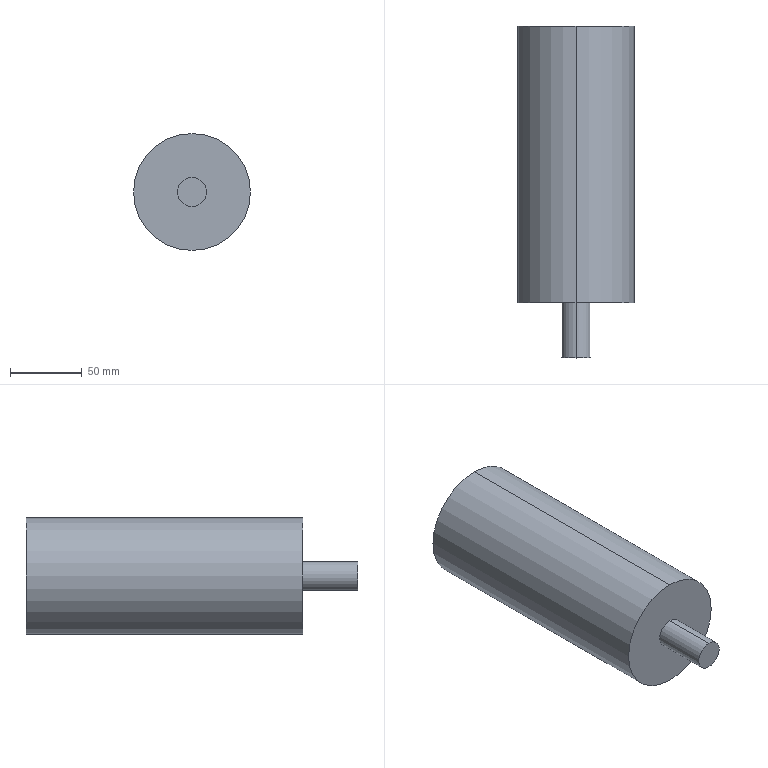Part | STEP file | 1 solid | 7 faces | box 81.521 x 231.5 x 81.521 mm | volume 1019717 mm3 | cylinder 4 | plane 3 | commonest cylinder face diameters 20.209 x2 81.521 x2
STEP:
#1=CARTESIAN_POINT('',(0.,0.,0.));
#2=DIRECTION('',(0.,0.,1.));
#3=DIRECTION('',(1.,0.,0.));
#4=AXIS2_PLACEMENT_3D('',#1,#2,#3);
#5=CARTESIAN_POINT('',(340.649,211.514,236.001));
#6=VERTEX_POINT('',#5);
#7=CARTESIAN_POINT('',(340.649,211.514,256.211));
#8=VERTEX_POINT('',#7);
#9=CARTESIAN_POINT('',(340.649,211.514,246.106));
#10=DIRECTION('',(0.,-1.,0.));
#11=DIRECTION('',(0.,0.,-1.));
#12=AXIS2_PLACEMENT_3D('',#9,#10,#11);
#13=CIRCLE('',#12,10.105);
#14=CARTESIAN_POINT('',(340.649,211.514,246.106));
#15=DIRECTION('',(0.,1.,0.));
#16=DIRECTION('',(0.,0.,1.));
#17=AXIS2_PLACEMENT_3D('',#14,#15,#16);
#18=CYLINDRICAL_SURFACE('',#17,10.105);
#19=CARTESIAN_POINT('',(3.142,0.));
#20=DIRECTION('',(-1.,0.));
#21=VECTOR('',#20,1.);
#22=LINE('',#19,#21);
#23=(GEOMETRIC_REPRESENTATION_CONTEXT(2)PARAMETRIC_REPRESENTATION_CONTEXT()REPRESENTATION_CONTEXT('',''));
#24=DEFINITIONAL_REPRESENTATION('',(#22),#23);
#25=PCURVE('',#18,#24);
#26=CARTESIAN_POINT('',(340.649,211.514,246.106));
#27=DIRECTION('',(0.,-1.,0.));
#28=DIRECTION('',(0.,0.,-1.));
#29=AXIS2_PLACEMENT_3D('',#26,#27,#28);
#30=PLANE('',#29);
#31=CARTESIAN_POINT('',(0.,0.));
#32=DIRECTION('',(1.,0.));
#33=AXIS2_PLACEMENT_2D('',#31,#32);
#34=CIRCLE('',#33,10.105);
#35=(GEOMETRIC_REPRESENTATION_CONTEXT(2)PARAMETRIC_REPRESENTATION_CONTEXT()REPRESENTATION_CONTEXT('',''));
#36=DEFINITIONAL_REPRESENTATION('',(#34),#35);
#37=PCURVE('',#30,#36);
#38=SURFACE_CURVE('',#13,(#25,#37),.PCURVE_S1.);
#39=EDGE_CURVE('',#6,#8,#38,.T.);
#40=ORIENTED_EDGE('',*,*,#39,.F.);
#41=CARTESIAN_POINT('',(340.649,250.014,236.001));
#42=VERTEX_POINT('',#41);
#43=CARTESIAN_POINT('',(340.649,211.514,236.001));
#44=DIRECTION('',(0.,1.,0.));
#45=VECTOR('',#44,1.);
#46=LINE('',#43,#45);
#47=CARTESIAN_POINT('',(3.142,0.));
#48=DIRECTION('',(0.,1.));
#49=VECTOR('',#48,1.);
#50=LINE('',#47,#49);
#51=(GEOMETRIC_REPRESENTATION_CONTEXT(2)PARAMETRIC_REPRESENTATION_CONTEXT()REPRESENTATION_CONTEXT('',''));
#52=DEFINITIONAL_REPRESENTATION('',(#50),#51);
#53=PCURVE('',#18,#52);
#54=CARTESIAN_POINT('',(340.649,211.514,246.106));
#55=DIRECTION('',(0.,1.,0.));
#56=DIRECTION('',(0.,0.,1.));
#57=AXIS2_PLACEMENT_3D('',#54,#55,#56);
#58=CYLINDRICAL_SURFACE('',#57,10.105);
#59=CARTESIAN_POINT('',(3.142,0.));
#60=DIRECTION('',(0.,1.));
#61=VECTOR('',#60,1.);
#62=LINE('',#59,#61);
#63=(GEOMETRIC_REPRESENTATION_CONTEXT(2)PARAMETRIC_REPRESENTATION_CONTEXT()REPRESENTATION_CONTEXT('',''));
#64=DEFINITIONAL_REPRESENTATION('',(#62),#63);
#65=PCURVE('',#58,#64);
#66=SURFACE_CURVE('',#46,(#53,#65),.PCURVE_S1.);
#67=EDGE_CURVE('',#6,#42,#66,.T.);
#68=ORIENTED_EDGE('',*,*,#67,.T.);
#69=CARTESIAN_POINT('',(340.649,250.014,256.211));
#70=VERTEX_POINT('',#69);
#71=CARTESIAN_POINT('',(340.649,250.014,246.106));
#72=DIRECTION('',(0.,-1.,0.));
#73=DIRECTION('',(0.,0.,1.));
#74=AXIS2_PLACEMENT_3D('',#71,#72,#73);
#75=CIRCLE('',#74,10.105);
#76=CARTESIAN_POINT('',(6.283,38.5));
#77=DIRECTION('',(-1.,0.));
#78=VECTOR('',#77,1.);
#79=LINE('',#76,#78);
#80=(GEOMETRIC_REPRESENTATION_CONTEXT(2)PARAMETRIC_REPRESENTATION_CONTEXT()REPRESENTATION_CONTEXT('',''));
#81=DEFINITIONAL_REPRESENTATION('',(#79),#80);
#82=PCURVE('',#18,#81);
#83=CARTESIAN_POINT('',(340.649,250.014,246.106));
#84=DIRECTION('',(0.,1.,0.));
#85=DIRECTION('',(0.,0.,1.));
#86=AXIS2_PLACEMENT_3D('',#83,#84,#85);
#87=PLANE('',#86);
#88=CARTESIAN_POINT('',(10.105,0.));
#89=CARTESIAN_POINT('',(10.105,-17.502));
#90=CARTESIAN_POINT('',(-5.052,-8.751));
#91=CARTESIAN_POINT('',(-20.209,0.));
#92=CARTESIAN_POINT('',(-5.052,8.751));
#93=CARTESIAN_POINT('',(10.105,17.502));
#94=CARTESIAN_POINT('',(10.105,0.));
#95=(BOUNDED_CURVE()B_SPLINE_CURVE(2,(#88,#89,#90,#91,#92,#93,#94),.UNSPECIFIED.,.T.,.F.)B_SPLINE_CURVE_WITH_KNOTS((1,2,2,2,2,1),(-2.094,0.,2.094,4.189,6.283,8.378),.UNSPECIFIED.)CURVE()GEOMETRIC_REPRESENTATION_ITEM()RATIONAL_B_SPLINE_CURVE((1.,0.5,1.,0.5,1.,0.5,1.))REPRESENTATION_ITEM(''));
#96=(GEOMETRIC_REPRESENTATION_CONTEXT(2)PARAMETRIC_REPRESENTATION_CONTEXT()REPRESENTATION_CONTEXT('',''));
#97=DEFINITIONAL_REPRESENTATION('',(#95),#96);
#98=PCURVE('',#87,#97);
#99=SURFACE_CURVE('',#75,(#82,#98),.PCURVE_S1.);
#100=EDGE_CURVE('',#42,#70,#99,.T.);
#101=ORIENTED_EDGE('',*,*,#100,.T.);
#102=CARTESIAN_POINT('',(340.649,211.514,256.211));
#103=DIRECTION('',(0.,1.,0.));
#104=VECTOR('',#103,1.);
#105=LINE('',#102,#104);
#106=CARTESIAN_POINT('',(0.,0.));
#107=DIRECTION('',(0.,1.));
#108=VECTOR('',#107,1.);
#109=LINE('',#106,#108);
#110=(GEOMETRIC_REPRESENTATION_CONTEXT(2)PARAMETRIC_REPRESENTATION_CONTEXT()REPRESENTATION_CONTEXT('',''));
#111=DEFINITIONAL_REPRESENTATION('',(#109),#110);
#112=PCURVE('',#18,#111);
#113=CARTESIAN_POINT('',(6.283,0.));
#114=DIRECTION('',(0.,1.));
#115=VECTOR('',#114,1.);
#116=LINE('',#113,#115);
#117=(GEOMETRIC_REPRESENTATION_CONTEXT(2)PARAMETRIC_REPRESENTATION_CONTEXT()REPRESENTATION_CONTEXT('',''));
#118=DEFINITIONAL_REPRESENTATION('',(#116),#117);
#119=PCURVE('',#58,#118);
#120=SURFACE_CURVE('',#105,(#112,#119),.PCURVE_S1.);
#121=EDGE_CURVE('',#8,#70,#120,.T.);
#122=ORIENTED_EDGE('',*,*,#121,.F.);
#123=EDGE_LOOP('',(#40,#68,#101,#122));
#124=FACE_BOUND('',#123,.T.);
#125=ADVANCED_FACE('',(#124),#18,.T.);
#126=CARTESIAN_POINT('',(340.649,443.014,286.866));
#127=VERTEX_POINT('',#126);
#128=CARTESIAN_POINT('',(340.649,443.014,205.345));
#129=VERTEX_POINT('',#128);
#130=CARTESIAN_POINT('',(340.649,443.014,246.106));
#131=DIRECTION('',(0.,1.,0.));
#132=DIRECTION('',(0.,0.,1.));
#133=AXIS2_PLACEMENT_3D('',#130,#131,#132);
#134=CIRCLE('',#133,40.761);
#135=CARTESIAN_POINT('',(340.649,443.014,246.106));
#136=DIRECTION('',(0.,-1.,0.));
#137=DIRECTION('',(0.,0.,-1.));
#138=AXIS2_PLACEMENT_3D('',#135,#136,#137);
#139=CYLINDRICAL_SURFACE('',#138,40.761);
#140=CARTESIAN_POINT('',(3.142,0.));
#141=DIRECTION('',(-1.,0.));
#142=VECTOR('',#141,1.);
#143=LINE('',#140,#142);
#144=(GEOMETRIC_REPRESENTATION_CONTEXT(2)PARAMETRIC_REPRESENTATION_CONTEXT()REPRESENTATION_CONTEXT('',''));
#145=DEFINITIONAL_REPRESENTATION('',(#143),#144);
#146=PCURVE('',#139,#145);
#147=CARTESIAN_POINT('',(340.649,443.014,246.106));
#148=DIRECTION('',(0.,1.,0.));
#149=DIRECTION('',(0.,0.,1.));
#150=AXIS2_PLACEMENT_3D('',#147,#148,#149);
#151=PLANE('',#150);
#152=CARTESIAN_POINT('',(0.,0.));
#153=DIRECTION('',(1.,0.));
#154=AXIS2_PLACEMENT_2D('',#152,#153);
#155=CIRCLE('',#154,40.761);
#156=(GEOMETRIC_REPRESENTATION_CONTEXT(2)PARAMETRIC_REPRESENTATION_CONTEXT()REPRESENTATION_CONTEXT('',''));
#157=DEFINITIONAL_REPRESENTATION('',(#155),#156);
#158=PCURVE('',#151,#157);
#159=SURFACE_CURVE('',#134,(#146,#158),.PCURVE_S1.);
#160=EDGE_CURVE('',#127,#129,#159,.T.);
#161=ORIENTED_EDGE('',*,*,#160,.F.);
#162=CARTESIAN_POINT('',(340.649,250.014,286.866));
#163=VERTEX_POINT('',#162);
#164=CARTESIAN_POINT('',(340.649,443.014,286.866));
#165=DIRECTION('',(0.,-1.,0.));
#166=VECTOR('',#165,1.);
#167=LINE('',#164,#166);
#168=CARTESIAN_POINT('',(3.142,0.));
#169=DIRECTION('',(0.,1.));
#170=VECTOR('',#169,1.);
#171=LINE('',#168,#170);
#172=(GEOMETRIC_REPRESENTATION_CONTEXT(2)PARAMETRIC_REPRESENTATION_CONTEXT()REPRESENTATION_CONTEXT('',''));
#173=DEFINITIONAL_REPRESENTATION('',(#171),#172);
#174=PCURVE('',#139,#173);
#175=CARTESIAN_POINT('',(340.649,443.014,246.106));
#176=DIRECTION('',(0.,-1.,0.));
#177=DIRECTION('',(0.,0.,-1.));
#178=AXIS2_PLACEMENT_3D('',#175,#176,#177);
#179=CYLINDRICAL_SURFACE('',#178,40.761);
#180=CARTESIAN_POINT('',(3.142,0.));
#181=DIRECTION('',(0.,1.));
#182=VECTOR('',#181,1.);
#183=LINE('',#180,#182);
#184=(GEOMETRIC_REPRESENTATION_CONTEXT(2)PARAMETRIC_REPRESENTATION_CONTEXT()REPRESENTATION_CONTEXT('',''));
#185=DEFINITIONAL_REPRESENTATION('',(#183),#184);
#186=PCURVE('',#179,#185);
#187=SURFACE_CURVE('',#167,(#174,#186),.PCURVE_S1.);
#188=EDGE_CURVE('',#127,#163,#187,.T.);
#189=ORIENTED_EDGE('',*,*,#188,.T.);
#190=CARTESIAN_POINT('',(340.649,250.014,205.345));
#191=VERTEX_POINT('',#190);
#192=CARTESIAN_POINT('',(340.649,250.014,246.106));
#193=DIRECTION('',(0.,1.,0.));
#194=DIRECTION('',(0.,0.,1.));
#195=AXIS2_PLACEMENT_3D('',#192,#193,#194);
#196=CIRCLE('',#195,40.761);
#197=CARTESIAN_POINT('',(3.142,193.));
#198=DIRECTION('',(-1.,0.));
#199=VECTOR('',#198,1.);
#200=LINE('',#197,#199);
#201=(GEOMETRIC_REPRESENTATION_CONTEXT(2)PARAMETRIC_REPRESENTATION_CONTEXT()REPRESENTATION_CONTEXT('',''));
#202=DEFINITIONAL_REPRESENTATION('',(#200),#201);
#203=PCURVE('',#139,#202);
#204=CARTESIAN_POINT('',(0.,0.));
#205=DIRECTION('',(1.,0.));
#206=AXIS2_PLACEMENT_2D('',#204,#205);
#207=CIRCLE('',#206,40.761);
#208=(GEOMETRIC_REPRESENTATION_CONTEXT(2)PARAMETRIC_REPRESENTATION_CONTEXT()REPRESENTATION_CONTEXT('',''));
#209=DEFINITIONAL_REPRESENTATION('',(#207),#208);
#210=PCURVE('',#87,#209);
#211=SURFACE_CURVE('',#196,(#203,#210),.PCURVE_S1.);
#212=EDGE_CURVE('',#163,#191,#211,.T.);
#213=ORIENTED_EDGE('',*,*,#212,.T.);
#214=CARTESIAN_POINT('',(340.649,443.014,205.345));
#215=DIRECTION('',(0.,-1.,0.));
#216=VECTOR('',#215,1.);
#217=LINE('',#214,#216);
#218=CARTESIAN_POINT('',(0.,0.));
#219=DIRECTION('',(0.,1.));
#220=VECTOR('',#219,1.);
#221=LINE('',#218,#220);
#222=(GEOMETRIC_REPRESENTATION_CONTEXT(2)PARAMETRIC_REPRESENTATION_CONTEXT()REPRESENTATION_CONTEXT('',''));
#223=DEFINITIONAL_REPRESENTATION('',(#221),#222);
#224=PCURVE('',#139,#223);
#225=CARTESIAN_POINT('',(6.283,0.));
#226=DIRECTION('',(0.,1.));
#227=VECTOR('',#226,1.);
#228=LINE('',#225,#227);
#229=(GEOMETRIC_REPRESENTATION_CONTEXT(2)PARAMETRIC_REPRESENTATION_CONTEXT()REPRESENTATION_CONTEXT('',''));
#230=DEFINITIONAL_REPRESENTATION('',(#228),#229);
#231=PCURVE('',#179,#230);
#232=SURFACE_CURVE('',#217,(#224,#231),.PCURVE_S1.);
#233=EDGE_CURVE('',#129,#191,#232,.T.);
#234=ORIENTED_EDGE('',*,*,#233,.F.);
#235=EDGE_LOOP('',(#161,#189,#213,#234));
#236=FACE_BOUND('',#235,.T.);
#237=ADVANCED_FACE('',(#236),#139,.T.);
#238=ORIENTED_EDGE('',*,*,#188,.F.);
#239=CARTESIAN_POINT('',(340.649,443.014,246.106));
#240=DIRECTION('',(0.,1.,0.));
#241=DIRECTION('',(0.,0.,1.));
#242=AXIS2_PLACEMENT_3D('',#239,#240,#241);
#243=CIRCLE('',#242,40.761);
#244=CARTESIAN_POINT('',(9.425,0.));
#245=DIRECTION('',(-1.,0.));
#246=VECTOR('',#245,1.);
#247=LINE('',#244,#246);
#248=(GEOMETRIC_REPRESENTATION_CONTEXT(2)PARAMETRIC_REPRESENTATION_CONTEXT()REPRESENTATION_CONTEXT('',''));
#249=DEFINITIONAL_REPRESENTATION('',(#247),#248);
#250=PCURVE('',#179,#249);
#251=CARTESIAN_POINT('',(0.,0.));
#252=DIRECTION('',(1.,0.));
#253=AXIS2_PLACEMENT_2D('',#251,#252);
#254=CIRCLE('',#253,40.761);
#255=(GEOMETRIC_REPRESENTATION_CONTEXT(2)PARAMETRIC_REPRESENTATION_CONTEXT()REPRESENTATION_CONTEXT('',''));
#256=DEFINITIONAL_REPRESENTATION('',(#254),#255);
#257=PCURVE('',#151,#256);
#258=SURFACE_CURVE('',#243,(#250,#257),.PCURVE_S1.);
#259=EDGE_CURVE('',#129,#127,#258,.T.);
#260=ORIENTED_EDGE('',*,*,#259,.F.);
#261=ORIENTED_EDGE('',*,*,#233,.T.);
#262=CARTESIAN_POINT('',(340.649,250.014,246.106));
#263=DIRECTION('',(0.,1.,0.));
#264=DIRECTION('',(0.,0.,1.));
#265=AXIS2_PLACEMENT_3D('',#262,#263,#264);
#266=CIRCLE('',#265,40.761);
#267=CARTESIAN_POINT('',(9.425,193.));
#268=DIRECTION('',(-1.,0.));
#269=VECTOR('',#268,1.);
#270=LINE('',#267,#269);
#271=(GEOMETRIC_REPRESENTATION_CONTEXT(2)PARAMETRIC_REPRESENTATION_CONTEXT()REPRESENTATION_CONTEXT('',''));
#272=DEFINITIONAL_REPRESENTATION('',(#270),#271);
#273=PCURVE('',#179,#272);
#274=CARTESIAN_POINT('',(0.,0.));
#275=DIRECTION('',(1.,0.));
#276=AXIS2_PLACEMENT_2D('',#274,#275);
#277=CIRCLE('',#276,40.761);
#278=(GEOMETRIC_REPRESENTATION_CONTEXT(2)PARAMETRIC_REPRESENTATION_CONTEXT()REPRESENTATION_CONTEXT('',''));
#279=DEFINITIONAL_REPRESENTATION('',(#277),#278);
#280=PCURVE('',#87,#279);
#281=SURFACE_CURVE('',#266,(#273,#280),.PCURVE_S1.);
#282=EDGE_CURVE('',#191,#163,#281,.T.);
#283=ORIENTED_EDGE('',*,*,#282,.T.);
#284=EDGE_LOOP('',(#238,#260,#261,#283));
#285=FACE_BOUND('',#284,.T.);
#286=ADVANCED_FACE('',(#285),#179,.T.);
#287=ORIENTED_EDGE('',*,*,#259,.T.);
#288=ORIENTED_EDGE('',*,*,#160,.T.);
#289=EDGE_LOOP('',(#287,#288));
#290=FACE_BOUND('',#289,.T.);
#291=ADVANCED_FACE('',(#290),#151,.T.);
#292=CARTESIAN_POINT('',(340.649,250.014,246.106));
#293=DIRECTION('',(0.,-1.,0.));
#294=DIRECTION('',(0.,0.,1.));
#295=AXIS2_PLACEMENT_3D('',#292,#293,#294);
#296=CIRCLE('',#295,10.105);
#297=CARTESIAN_POINT('',(10.105,0.));
#298=CARTESIAN_POINT('',(10.105,-17.502));
#299=CARTESIAN_POINT('',(-5.052,-8.751));
#300=CARTESIAN_POINT('',(-20.209,0.));
#301=CARTESIAN_POINT('',(-5.052,8.751));
#302=CARTESIAN_POINT('',(10.105,17.502));
#303=CARTESIAN_POINT('',(10.105,0.));
#304=(BOUNDED_CURVE()B_SPLINE_CURVE(2,(#297,#298,#299,#300,#301,#302,#303),.UNSPECIFIED.,.T.,.F.)B_SPLINE_CURVE_WITH_KNOTS((1,2,2,2,2,1),(-2.094,0.,2.094,4.189,6.283,8.378),.UNSPECIFIED.)CURVE()GEOMETRIC_REPRESENTATION_ITEM()RATIONAL_B_SPLINE_CURVE((1.,0.5,1.,0.5,1.,0.5,1.))REPRESENTATION_ITEM(''));
#305=(GEOMETRIC_REPRESENTATION_CONTEXT(2)PARAMETRIC_REPRESENTATION_CONTEXT()REPRESENTATION_CONTEXT('',''));
#306=DEFINITIONAL_REPRESENTATION('',(#304),#305);
#307=PCURVE('',#87,#306);
#308=CARTESIAN_POINT('',(6.283,38.5));
#309=DIRECTION('',(-1.,0.));
#310=VECTOR('',#309,1.);
#311=LINE('',#308,#310);
#312=(GEOMETRIC_REPRESENTATION_CONTEXT(2)PARAMETRIC_REPRESENTATION_CONTEXT()REPRESENTATION_CONTEXT('',''));
#313=DEFINITIONAL_REPRESENTATION('',(#311),#312);
#314=PCURVE('',#58,#313);
#315=SURFACE_CURVE('',#296,(#307,#314),.PCURVE_S1.);
#316=EDGE_CURVE('',#70,#42,#315,.T.);
#317=ORIENTED_EDGE('',*,*,#316,.F.);
#318=ORIENTED_EDGE('',*,*,#100,.F.);
#319=EDGE_LOOP('',(#317,#318));
#320=FACE_BOUND('',#319,.T.);
#321=ORIENTED_EDGE('',*,*,#282,.F.);
#322=ORIENTED_EDGE('',*,*,#212,.F.);
#323=EDGE_LOOP('',(#321,#322));
#324=FACE_BOUND('',#323,.T.);
#325=ADVANCED_FACE('',(#320,#324),#87,.F.);
#326=ORIENTED_EDGE('',*,*,#67,.F.);
#327=CARTESIAN_POINT('',(340.649,211.514,246.106));
#328=DIRECTION('',(0.,-1.,0.));
#329=DIRECTION('',(0.,0.,-1.));
#330=AXIS2_PLACEMENT_3D('',#327,#328,#329);
#331=CIRCLE('',#330,10.105);
#332=CARTESIAN_POINT('',(9.425,0.));
#333=DIRECTION('',(-1.,0.));
#334=VECTOR('',#333,1.);
#335=LINE('',#332,#334);
#336=(GEOMETRIC_REPRESENTATION_CONTEXT(2)PARAMETRIC_REPRESENTATION_CONTEXT()REPRESENTATION_CONTEXT('',''));
#337=DEFINITIONAL_REPRESENTATION('',(#335),#336);
#338=PCURVE('',#58,#337);
#339=CARTESIAN_POINT('',(0.,0.));
#340=DIRECTION('',(1.,0.));
#341=AXIS2_PLACEMENT_2D('',#339,#340);
#342=CIRCLE('',#341,10.105);
#343=(GEOMETRIC_REPRESENTATION_CONTEXT(2)PARAMETRIC_REPRESENTATION_CONTEXT()REPRESENTATION_CONTEXT('',''));
#344=DEFINITIONAL_REPRESENTATION('',(#342),#343);
#345=PCURVE('',#30,#344);
#346=SURFACE_CURVE('',#331,(#338,#345),.PCURVE_S1.);
#347=EDGE_CURVE('',#8,#6,#346,.T.);
#348=ORIENTED_EDGE('',*,*,#347,.F.);
#349=ORIENTED_EDGE('',*,*,#121,.T.);
#350=ORIENTED_EDGE('',*,*,#316,.T.);
#351=EDGE_LOOP('',(#326,#348,#349,#350));
#352=FACE_BOUND('',#351,.T.);
#353=ADVANCED_FACE('',(#352),#58,.T.);
#354=ORIENTED_EDGE('',*,*,#347,.T.);
#355=ORIENTED_EDGE('',*,*,#39,.T.);
#356=EDGE_LOOP('',(#354,#355));
#357=FACE_BOUND('',#356,.T.);
#358=ADVANCED_FACE('',(#357),#30,.T.);
#359=CLOSED_SHELL('',(#125,#237,#286,#291,#325,#353,#358));
#360=MANIFOLD_SOLID_BREP('',#359);
#361=(LENGTH_UNIT()NAMED_UNIT(*)SI_UNIT(.MILLI.,.METRE.));
#362=UNCERTAINTY_MEASURE_WITH_UNIT(LENGTH_MEASURE(0.0000001),#361,'','');
#363=(NAMED_UNIT(*)PLANE_ANGLE_UNIT()SI_UNIT($,.RADIAN.));
#364=(NAMED_UNIT(*)SI_UNIT($,.STERADIAN.)SOLID_ANGLE_UNIT());
#365=(GEOMETRIC_REPRESENTATION_CONTEXT(3)GLOBAL_UNCERTAINTY_ASSIGNED_CONTEXT((#362))GLOBAL_UNIT_ASSIGNED_CONTEXT((#361,#363,#364))REPRESENTATION_CONTEXT('',''));
#366=ADVANCED_BREP_SHAPE_REPRESENTATION('',(#4,#360),#365);